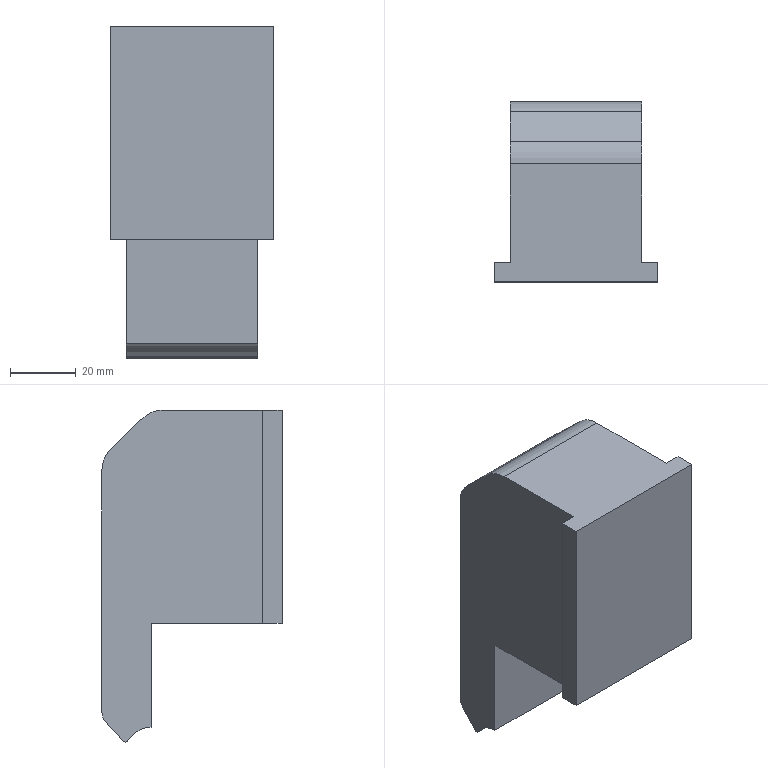Part | SolidWorks | features ICE 3, Extrusion 1, Fillet 1 | 1 solid | 21 faces | box 50 x 55 x 101.25 mm | volume 146000 mm3 | plane 14 | cylinder 7 | commonest cylinder face diameters 20 x2 21 x2 2 x1 10 x1 16.4 x1
STEP:
#1=CARTESIAN_POINT('',(10.5,25.,14.5));
#2=VERTEX_POINT('',#1);
#3=CARTESIAN_POINT('',(-10.5,25.,14.5));
#4=VERTEX_POINT('',#3);
#5=CARTESIAN_POINT('',(0.,25.,14.5));
#6=DIRECTION('',(0.,0.,-1.));
#7=DIRECTION('',(-1.,0.,0.));
#8=AXIS2_PLACEMENT_3D('',#5,#6,#7);
#9=CIRCLE('',#8,10.5);
#10=EDGE_CURVE('',#2,#4,#9,.T.);
#11=ORIENTED_EDGE('',*,*,#10,.F.);
#12=CARTESIAN_POINT('',(10.5,25.,-32.5));
#13=VERTEX_POINT('',#12);
#14=CARTESIAN_POINT('',(10.5,25.,14.5));
#15=DIRECTION('',(0.,0.,-1.));
#16=VECTOR('',#15,1000.);
#17=LINE('',#14,#16);
#18=EDGE_CURVE('',#2,#13,#17,.T.);
#19=ORIENTED_EDGE('',*,*,#18,.T.);
#20=CARTESIAN_POINT('',(-10.5,25.,-32.5));
#21=VERTEX_POINT('',#20);
#22=CARTESIAN_POINT('',(0.,25.,-32.5));
#23=DIRECTION('',(0.,0.,-1.));
#24=DIRECTION('',(-1.,0.,0.));
#25=AXIS2_PLACEMENT_3D('',#22,#23,#24);
#26=CIRCLE('',#25,10.5);
#27=EDGE_CURVE('',#13,#21,#26,.T.);
#28=ORIENTED_EDGE('',*,*,#27,.T.);
#29=CARTESIAN_POINT('',(-10.5,25.,14.5));
#30=DIRECTION('',(0.,0.,-1.));
#31=VECTOR('',#30,1000.);
#32=LINE('',#29,#31);
#33=EDGE_CURVE('',#4,#21,#32,.T.);
#34=ORIENTED_EDGE('',*,*,#33,.F.);
#35=EDGE_LOOP('',(#11,#19,#28,#34));
#36=FACE_OUTER_BOUND('',#35,.T.);
#37=CARTESIAN_POINT('',(0.,25.,14.5));
#38=DIRECTION('',(0.,0.,-1.));
#39=DIRECTION('',(-1.,0.,0.));
#40=AXIS2_PLACEMENT_3D('',#37,#38,#39);
#41=CYLINDRICAL_SURFACE('',#40,10.5);
#42=ADVANCED_FACE('',(#36),#41,.F.);
#43=CARTESIAN_POINT('',(20.,6.,32.5));
#44=VERTEX_POINT('',#43);
#45=CARTESIAN_POINT('',(20.,6.,-32.5));
#46=VERTEX_POINT('',#45);
#47=CARTESIAN_POINT('',(20.,6.,-32.5));
#48=DIRECTION('',(0.,0.,-1.));
#49=VECTOR('',#48,1000.);
#50=LINE('',#47,#49);
#51=EDGE_CURVE('',#44,#46,#50,.T.);
#52=ORIENTED_EDGE('',*,*,#51,.F.);
#53=CARTESIAN_POINT('',(25.,6.,32.5));
#54=VERTEX_POINT('',#53);
#55=CARTESIAN_POINT('',(-25.,6.,32.5));
#56=DIRECTION('',(1.,0.,0.));
#57=VECTOR('',#56,1000.);
#58=LINE('',#55,#57);
#59=EDGE_CURVE('',#44,#54,#58,.T.);
#60=ORIENTED_EDGE('',*,*,#59,.T.);
#61=CARTESIAN_POINT('',(25.,6.,-32.5));
#62=VERTEX_POINT('',#61);
#63=CARTESIAN_POINT('',(25.,6.,32.5));
#64=DIRECTION('',(0.,0.,-1.));
#65=VECTOR('',#64,1000.);
#66=LINE('',#63,#65);
#67=EDGE_CURVE('',#54,#62,#66,.T.);
#68=ORIENTED_EDGE('',*,*,#67,.T.);
#69=CARTESIAN_POINT('',(-25.,6.,-32.5));
#70=DIRECTION('',(-1.,0.,0.));
#71=VECTOR('',#70,1000.);
#72=LINE('',#69,#71);
#73=EDGE_CURVE('',#62,#46,#72,.T.);
#74=ORIENTED_EDGE('',*,*,#73,.T.);
#75=EDGE_LOOP('',(#52,#60,#68,#74));
#76=FACE_OUTER_BOUND('',#75,.T.);
#77=CARTESIAN_POINT('',(0.,6.,0.));
#78=DIRECTION('',(0.,-1.,0.));
#79=DIRECTION('',(0.,0.,-1.));
#80=AXIS2_PLACEMENT_3D('',#77,#78,#79);
#81=PLANE('',#80);
#82=ADVANCED_FACE('',(#76),#81,.F.);
#83=CARTESIAN_POINT('',(-20.,6.,-32.5));
#84=VERTEX_POINT('',#83);
#85=CARTESIAN_POINT('',(-20.,6.,32.5));
#86=VERTEX_POINT('',#85);
#87=CARTESIAN_POINT('',(-20.,6.,-32.5));
#88=DIRECTION('',(0.,0.,1.));
#89=VECTOR('',#88,1000.);
#90=LINE('',#87,#89);
#91=EDGE_CURVE('',#84,#86,#90,.T.);
#92=ORIENTED_EDGE('',*,*,#91,.F.);
#93=CARTESIAN_POINT('',(-25.,6.,-32.5));
#94=VERTEX_POINT('',#93);
#95=CARTESIAN_POINT('',(-25.,6.,-32.5));
#96=DIRECTION('',(-1.,0.,0.));
#97=VECTOR('',#96,1000.);
#98=LINE('',#95,#97);
#99=EDGE_CURVE('',#84,#94,#98,.T.);
#100=ORIENTED_EDGE('',*,*,#99,.T.);
#101=CARTESIAN_POINT('',(-25.,6.,32.5));
#102=VERTEX_POINT('',#101);
#103=CARTESIAN_POINT('',(-25.,6.,32.5));
#104=DIRECTION('',(0.,0.,1.));
#105=VECTOR('',#104,1000.);
#106=LINE('',#103,#105);
#107=EDGE_CURVE('',#94,#102,#106,.T.);
#108=ORIENTED_EDGE('',*,*,#107,.T.);
#109=CARTESIAN_POINT('',(-25.,6.,32.5));
#110=DIRECTION('',(1.,0.,0.));
#111=VECTOR('',#110,1000.);
#112=LINE('',#109,#111);
#113=EDGE_CURVE('',#102,#86,#112,.T.);
#114=ORIENTED_EDGE('',*,*,#113,.T.);
#115=EDGE_LOOP('',(#92,#100,#108,#114));
#116=FACE_OUTER_BOUND('',#115,.T.);
#117=CARTESIAN_POINT('',(0.,6.,0.));
#118=DIRECTION('',(0.,-1.,0.));
#119=DIRECTION('',(0.,0.,-1.));
#120=AXIS2_PLACEMENT_3D('',#117,#118,#119);
#121=PLANE('',#120);
#122=ADVANCED_FACE('',(#116),#121,.F.);
#123=CARTESIAN_POINT('',(25.,0.,32.5));
#124=VERTEX_POINT('',#123);
#125=CARTESIAN_POINT('',(25.,0.,-32.5));
#126=VERTEX_POINT('',#125);
#127=CARTESIAN_POINT('',(25.,0.,32.5));
#128=DIRECTION('',(0.,0.,-1.));
#129=VECTOR('',#128,1000.);
#130=LINE('',#127,#129);
#131=EDGE_CURVE('',#124,#126,#130,.T.);
#132=ORIENTED_EDGE('',*,*,#131,.T.);
#133=CARTESIAN_POINT('',(25.,6.,-32.5));
#134=DIRECTION('',(0.,-1.,0.));
#135=VECTOR('',#134,1000.);
#136=LINE('',#133,#135);
#137=EDGE_CURVE('',#62,#126,#136,.T.);
#138=ORIENTED_EDGE('',*,*,#137,.F.);
#139=ORIENTED_EDGE('',*,*,#67,.F.);
#140=CARTESIAN_POINT('',(25.,6.,32.5));
#141=DIRECTION('',(0.,-1.,0.));
#142=VECTOR('',#141,1000.);
#143=LINE('',#140,#142);
#144=EDGE_CURVE('',#54,#124,#143,.T.);
#145=ORIENTED_EDGE('',*,*,#144,.T.);
#146=EDGE_LOOP('',(#132,#138,#139,#145));
#147=FACE_OUTER_BOUND('',#146,.T.);
#148=CARTESIAN_POINT('',(25.,6.,32.5));
#149=DIRECTION('',(-1.,0.,0.));
#150=DIRECTION('',(0.,0.,1.));
#151=AXIS2_PLACEMENT_3D('',#148,#149,#150);
#152=PLANE('',#151);
#153=ADVANCED_FACE('',(#147),#152,.F.);
#154=CARTESIAN_POINT('',(0.,25.,-32.5));
#155=DIRECTION('',(0.,0.,-1.));
#156=DIRECTION('',(-1.,0.,0.));
#157=AXIS2_PLACEMENT_3D('',#154,#155,#156);
#158=CIRCLE('',#157,10.5);
#159=EDGE_CURVE('',#21,#13,#158,.T.);
#160=ORIENTED_EDGE('',*,*,#159,.F.);
#161=ORIENTED_EDGE('',*,*,#27,.F.);
#162=EDGE_LOOP('',(#160,#161));
#163=FACE_BOUND('',#162,.T.);
#164=CARTESIAN_POINT('',(-25.,0.,-32.5));
#165=VERTEX_POINT('',#164);
#166=CARTESIAN_POINT('',(-25.,0.,-32.5));
#167=DIRECTION('',(-1.,0.,0.));
#168=VECTOR('',#167,1000.);
#169=LINE('',#166,#168);
#170=EDGE_CURVE('',#126,#165,#169,.T.);
#171=ORIENTED_EDGE('',*,*,#170,.T.);
#172=CARTESIAN_POINT('',(-25.,6.,-32.5));
#173=DIRECTION('',(0.,-1.,0.));
#174=VECTOR('',#173,1000.);
#175=LINE('',#172,#174);
#176=EDGE_CURVE('',#94,#165,#175,.T.);
#177=ORIENTED_EDGE('',*,*,#176,.F.);
#178=ORIENTED_EDGE('',*,*,#99,.F.);
#179=CARTESIAN_POINT('',(-20.,40.,-32.5));
#180=VERTEX_POINT('',#179);
#181=CARTESIAN_POINT('',(-20.,40.,-32.5));
#182=DIRECTION('',(0.,-1.,0.));
#183=VECTOR('',#182,1000.);
#184=LINE('',#181,#183);
#185=EDGE_CURVE('',#180,#84,#184,.T.);
#186=ORIENTED_EDGE('',*,*,#185,.F.);
#187=CARTESIAN_POINT('',(20.,40.,-32.5));
#188=VERTEX_POINT('',#187);
#189=CARTESIAN_POINT('',(-20.,40.,-32.5));
#190=DIRECTION('',(-1.,0.,0.));
#191=VECTOR('',#190,1000.);
#192=LINE('',#189,#191);
#193=EDGE_CURVE('',#188,#180,#192,.T.);
#194=ORIENTED_EDGE('',*,*,#193,.F.);
#195=CARTESIAN_POINT('',(20.,40.,-32.5));
#196=DIRECTION('',(0.,-1.,0.));
#197=VECTOR('',#196,1000.);
#198=LINE('',#195,#197);
#199=EDGE_CURVE('',#188,#46,#198,.T.);
#200=ORIENTED_EDGE('',*,*,#199,.T.);
#201=ORIENTED_EDGE('',*,*,#73,.F.);
#202=ORIENTED_EDGE('',*,*,#137,.T.);
#203=EDGE_LOOP('',(#171,#177,#178,#186,#194,#200,#201,#202));
#204=FACE_OUTER_BOUND('',#203,.T.);
#205=CARTESIAN_POINT('',(-25.,6.,-32.5));
#206=DIRECTION('',(0.,0.,1.));
#207=DIRECTION('',(1.,0.,0.));
#208=AXIS2_PLACEMENT_3D('',#205,#206,#207);
#209=PLANE('',#208);
#210=ADVANCED_FACE('',(#163,#204),#209,.F.);
#211=CARTESIAN_POINT('',(-25.,0.,32.5));
#212=VERTEX_POINT('',#211);
#213=CARTESIAN_POINT('',(-25.,0.,32.5));
#214=DIRECTION('',(0.,0.,1.));
#215=VECTOR('',#214,1000.);
#216=LINE('',#213,#215);
#217=EDGE_CURVE('',#165,#212,#216,.T.);
#218=ORIENTED_EDGE('',*,*,#217,.T.);
#219=CARTESIAN_POINT('',(-25.,6.,32.5));
#220=DIRECTION('',(0.,-1.,0.));
#221=VECTOR('',#220,1000.);
#222=LINE('',#219,#221);
#223=EDGE_CURVE('',#102,#212,#222,.T.);
#224=ORIENTED_EDGE('',*,*,#223,.F.);
#225=ORIENTED_EDGE('',*,*,#107,.F.);
#226=ORIENTED_EDGE('',*,*,#176,.T.);
#227=EDGE_LOOP('',(#218,#224,#225,#226));
#228=FACE_OUTER_BOUND('',#227,.T.);
#229=CARTESIAN_POINT('',(-25.,6.,32.5));
#230=DIRECTION('',(1.,0.,0.));
#231=DIRECTION('',(0.,0.,-1.));
#232=AXIS2_PLACEMENT_3D('',#229,#230,#231);
#233=PLANE('',#232);
#234=ADVANCED_FACE('',(#228),#233,.F.);
#235=CARTESIAN_POINT('',(20.,36.004,32.5));
#236=VERTEX_POINT('',#235);
#237=CARTESIAN_POINT('',(20.,40.,32.5));
#238=DIRECTION('',(0.,-1.,0.));
#239=VECTOR('',#238,1000.);
#240=LINE('',#237,#239);
#241=EDGE_CURVE('',#236,#44,#240,.T.);
#242=ORIENTED_EDGE('',*,*,#241,.F.);
#243=CARTESIAN_POINT('',(-20.,36.004,32.5));
#244=VERTEX_POINT('',#243);
#245=CARTESIAN_POINT('',(-25.,36.004,32.5));
#246=DIRECTION('',(-1.,0.,0.));
#247=VECTOR('',#246,1000.);
#248=LINE('',#245,#247);
#249=EDGE_CURVE('',#236,#244,#248,.T.);
#250=ORIENTED_EDGE('',*,*,#249,.T.);
#251=CARTESIAN_POINT('',(-20.,40.,32.5));
#252=DIRECTION('',(0.,-1.,0.));
#253=VECTOR('',#252,1000.);
#254=LINE('',#251,#253);
#255=EDGE_CURVE('',#244,#86,#254,.T.);
#256=ORIENTED_EDGE('',*,*,#255,.T.);
#257=ORIENTED_EDGE('',*,*,#113,.F.);
#258=ORIENTED_EDGE('',*,*,#223,.T.);
#259=CARTESIAN_POINT('',(-25.,0.,32.5));
#260=DIRECTION('',(1.,0.,0.));
#261=VECTOR('',#260,1000.);
#262=LINE('',#259,#261);
#263=EDGE_CURVE('',#212,#124,#262,.T.);
#264=ORIENTED_EDGE('',*,*,#263,.T.);
#265=ORIENTED_EDGE('',*,*,#144,.F.);
#266=ORIENTED_EDGE('',*,*,#59,.F.);
#267=EDGE_LOOP('',(#242,#250,#256,#257,#258,#264,#265,#266));
#268=FACE_OUTER_BOUND('',#267,.T.);
#269=CARTESIAN_POINT('',(-25.,6.,32.5));
#270=DIRECTION('',(0.,0.,-1.));
#271=DIRECTION('',(-1.,0.,0.));
#272=AXIS2_PLACEMENT_3D('',#269,#270,#271);
#273=PLANE('',#272);
#274=ADVANCED_FACE('',(#268),#273,.F.);
#275=ORIENTED_EDGE('',*,*,#131,.F.);
#276=ORIENTED_EDGE('',*,*,#263,.F.);
#277=ORIENTED_EDGE('',*,*,#217,.F.);
#278=ORIENTED_EDGE('',*,*,#170,.F.);
#279=EDGE_LOOP('',(#275,#276,#277,#278));
#280=FACE_OUTER_BOUND('',#279,.T.);
#281=CARTESIAN_POINT('',(0.,0.,0.));
#282=DIRECTION('',(0.,-1.,0.));
#283=DIRECTION('',(0.,0.,-1.));
#284=AXIS2_PLACEMENT_3D('',#281,#282,#283);
#285=PLANE('',#284);
#286=ADVANCED_FACE('',(#280),#285,.T.);
#287=CARTESIAN_POINT('',(20.,55.,-59.535));
#288=VERTEX_POINT('',#287);
#289=CARTESIAN_POINT('',(20.,55.,13.946));
#290=VERTEX_POINT('',#289);
#291=CARTESIAN_POINT('',(20.,55.,-28.363));
#292=DIRECTION('',(0.,0.,1.));
#293=VECTOR('',#292,1000.);
#294=LINE('',#291,#293);
#295=EDGE_CURVE('',#288,#290,#294,.T.);
#296=ORIENTED_EDGE('',*,*,#295,.T.);
#297=CARTESIAN_POINT('',(20.,51.891,21.192));
#298=VERTEX_POINT('',#297);
#299=CARTESIAN_POINT('',(20.,45.,13.946));
#300=DIRECTION('',(1.,0.,0.));
#301=DIRECTION('',(0.,0.,1.));
#302=AXIS2_PLACEMENT_3D('',#299,#300,#301);
#303=CIRCLE('',#302,10.);
#304=EDGE_CURVE('',#290,#298,#303,.T.);
#305=ORIENTED_EDGE('',*,*,#304,.T.);
#306=CARTESIAN_POINT('',(20.,42.895,29.747));
#307=VERTEX_POINT('',#306);
#308=CARTESIAN_POINT('',(20.,55.,18.236));
#309=DIRECTION('',(0.,-0.7247,0.6891));
#310=VECTOR('',#309,1000.);
#311=LINE('',#308,#310);
#312=EDGE_CURVE('',#298,#307,#311,.T.);
#313=ORIENTED_EDGE('',*,*,#312,.T.);
#314=CARTESIAN_POINT('',(20.,36.004,22.5));
#315=DIRECTION('',(1.,0.,0.));
#316=DIRECTION('',(0.,0.,1.));
#317=AXIS2_PLACEMENT_3D('',#314,#315,#316);
#318=CIRCLE('',#317,10.);
#319=EDGE_CURVE('',#307,#236,#318,.T.);
#320=ORIENTED_EDGE('',*,*,#319,.T.);
#321=ORIENTED_EDGE('',*,*,#241,.T.);
#322=ORIENTED_EDGE('',*,*,#51,.T.);
#323=ORIENTED_EDGE('',*,*,#199,.F.);
#324=CARTESIAN_POINT('',(20.,40.,-64.3));
#325=VERTEX_POINT('',#324);
#326=CARTESIAN_POINT('',(20.,40.,32.5));
#327=DIRECTION('',(0.,0.,-1.));
#328=VECTOR('',#327,1000.);
#329=LINE('',#326,#328);
#330=EDGE_CURVE('',#188,#325,#329,.T.);
#331=ORIENTED_EDGE('',*,*,#330,.T.);
#332=CARTESIAN_POINT('',(20.,47.023,-68.266));
#333=VERTEX_POINT('',#332);
#334=CARTESIAN_POINT('',(20.,40.,-72.5));
#335=DIRECTION('',(-1.,0.,0.));
#336=DIRECTION('',(0.,0.,1.));
#337=AXIS2_PLACEMENT_3D('',#334,#335,#336);
#338=CIRCLE('',#337,8.2);
#339=EDGE_CURVE('',#325,#333,#338,.T.);
#340=ORIENTED_EDGE('',*,*,#339,.T.);
#341=CARTESIAN_POINT('',(20.,48.615,-68.427));
#342=VERTEX_POINT('',#341);
#343=CARTESIAN_POINT('',(20.,47.879,-67.75));
#344=DIRECTION('',(1.,0.,0.));
#345=DIRECTION('',(0.,0.,-1.));
#346=AXIS2_PLACEMENT_3D('',#343,#344,#345);
#347=CIRCLE('',#346,1.);
#348=EDGE_CURVE('',#333,#342,#347,.T.);
#349=ORIENTED_EDGE('',*,*,#348,.T.);
#350=CARTESIAN_POINT('',(20.,53.68,-62.92));
#351=VERTEX_POINT('',#350);
#352=CARTESIAN_POINT('',(20.,53.68,-62.92));
#353=DIRECTION('',(0.,0.677,0.736));
#354=VECTOR('',#353,1000.);
#355=LINE('',#352,#354);
#356=EDGE_CURVE('',#342,#351,#355,.T.);
#357=ORIENTED_EDGE('',*,*,#356,.T.);
#358=CARTESIAN_POINT('',(20.,50.,-59.535));
#359=DIRECTION('',(1.,0.,0.));
#360=DIRECTION('',(0.,0.,1.));
#361=AXIS2_PLACEMENT_3D('',#358,#359,#360);
#362=CIRCLE('',#361,5.);
#363=EDGE_CURVE('',#351,#288,#362,.T.);
#364=ORIENTED_EDGE('',*,*,#363,.T.);
#365=EDGE_LOOP('',(#296,#305,#313,#320,#321,#322,#323,#331,#340,#349,#357,#364));
#366=FACE_OUTER_BOUND('',#365,.T.);
#367=CARTESIAN_POINT('',(20.,40.,-32.5));
#368=DIRECTION('',(-1.,0.,0.));
#369=DIRECTION('',(0.,0.,1.));
#370=AXIS2_PLACEMENT_3D('',#367,#368,#369);
#371=PLANE('',#370);
#372=ADVANCED_FACE('',(#366),#371,.F.);
#373=CARTESIAN_POINT('',(-20.,51.891,21.192));
#374=VERTEX_POINT('',#373);
#375=CARTESIAN_POINT('',(-20.,42.895,29.747));
#376=VERTEX_POINT('',#375);
#377=CARTESIAN_POINT('',(-20.,55.,18.236));
#378=DIRECTION('',(0.,-0.7247,0.6891));
#379=VECTOR('',#378,1000.);
#380=LINE('',#377,#379);
#381=EDGE_CURVE('',#374,#376,#380,.T.);
#382=ORIENTED_EDGE('',*,*,#381,.F.);
#383=CARTESIAN_POINT('',(-20.,55.,13.946));
#384=VERTEX_POINT('',#383);
#385=CARTESIAN_POINT('',(-20.,45.,13.946));
#386=DIRECTION('',(-1.,0.,0.));
#387=DIRECTION('',(0.,0.,-1.));
#388=AXIS2_PLACEMENT_3D('',#385,#386,#387);
#389=CIRCLE('',#388,10.);
#390=EDGE_CURVE('',#374,#384,#389,.T.);
#391=ORIENTED_EDGE('',*,*,#390,.T.);
#392=CARTESIAN_POINT('',(-20.,55.,-59.535));
#393=VERTEX_POINT('',#392);
#394=CARTESIAN_POINT('',(-20.,55.,-28.363));
#395=DIRECTION('',(0.,0.,1.));
#396=VECTOR('',#395,1000.);
#397=LINE('',#394,#396);
#398=EDGE_CURVE('',#393,#384,#397,.T.);
#399=ORIENTED_EDGE('',*,*,#398,.F.);
#400=CARTESIAN_POINT('',(-20.,53.68,-62.92));
#401=VERTEX_POINT('',#400);
#402=CARTESIAN_POINT('',(-20.,50.,-59.535));
#403=DIRECTION('',(1.,0.,0.));
#404=DIRECTION('',(0.,0.,1.));
#405=AXIS2_PLACEMENT_3D('',#402,#403,#404);
#406=CIRCLE('',#405,5.);
#407=EDGE_CURVE('',#401,#393,#406,.T.);
#408=ORIENTED_EDGE('',*,*,#407,.F.);
#409=CARTESIAN_POINT('',(-20.,48.615,-68.427));
#410=VERTEX_POINT('',#409);
#411=CARTESIAN_POINT('',(-20.,53.68,-62.92));
#412=DIRECTION('',(0.,0.677,0.736));
#413=VECTOR('',#412,1000.);
#414=LINE('',#411,#413);
#415=EDGE_CURVE('',#410,#401,#414,.T.);
#416=ORIENTED_EDGE('',*,*,#415,.F.);
#417=CARTESIAN_POINT('',(-20.,47.023,-68.266));
#418=VERTEX_POINT('',#417);
#419=CARTESIAN_POINT('',(-20.,47.879,-67.75));
#420=DIRECTION('',(1.,0.,0.));
#421=DIRECTION('',(0.,0.,-1.));
#422=AXIS2_PLACEMENT_3D('',#419,#420,#421);
#423=CIRCLE('',#422,1.);
#424=EDGE_CURVE('',#418,#410,#423,.T.);
#425=ORIENTED_EDGE('',*,*,#424,.F.);
#426=CARTESIAN_POINT('',(-20.,40.,-64.3));
#427=VERTEX_POINT('',#426);
#428=CARTESIAN_POINT('',(-20.,40.,-72.5));
#429=DIRECTION('',(-1.,0.,0.));
#430=DIRECTION('',(0.,0.,1.));
#431=AXIS2_PLACEMENT_3D('',#428,#429,#430);
#432=CIRCLE('',#431,8.2);
#433=EDGE_CURVE('',#427,#418,#432,.T.);
#434=ORIENTED_EDGE('',*,*,#433,.F.);
#435=CARTESIAN_POINT('',(-20.,40.,32.5));
#436=DIRECTION('',(0.,0.,-1.));
#437=VECTOR('',#436,1000.);
#438=LINE('',#435,#437);
#439=EDGE_CURVE('',#180,#427,#438,.T.);
#440=ORIENTED_EDGE('',*,*,#439,.F.);
#441=ORIENTED_EDGE('',*,*,#185,.T.);
#442=ORIENTED_EDGE('',*,*,#91,.T.);
#443=ORIENTED_EDGE('',*,*,#255,.F.);
#444=CARTESIAN_POINT('',(-20.,36.004,22.5));
#445=DIRECTION('',(-1.,0.,0.));
#446=DIRECTION('',(0.,0.,-1.));
#447=AXIS2_PLACEMENT_3D('',#444,#445,#446);
#448=CIRCLE('',#447,10.);
#449=EDGE_CURVE('',#244,#376,#448,.T.);
#450=ORIENTED_EDGE('',*,*,#449,.T.);
#451=EDGE_LOOP('',(#382,#391,#399,#408,#416,#425,#434,#440,#441,#442,#443,#450));
#452=FACE_OUTER_BOUND('',#451,.T.);
#453=CARTESIAN_POINT('',(-20.,40.,-32.5));
#454=DIRECTION('',(1.,0.,0.));
#455=DIRECTION('',(0.,0.,-1.));
#456=AXIS2_PLACEMENT_3D('',#453,#454,#455);
#457=PLANE('',#456);
#458=ADVANCED_FACE('',(#452),#457,.F.);
#459=ORIENTED_EDGE('',*,*,#18,.F.);
#460=CARTESIAN_POINT('',(0.,25.,14.5));
#461=DIRECTION('',(0.,0.,-1.));
#462=DIRECTION('',(-1.,0.,0.));
#463=AXIS2_PLACEMENT_3D('',#460,#461,#462);
#464=CIRCLE('',#463,10.5);
#465=EDGE_CURVE('',#4,#2,#464,.T.);
#466=ORIENTED_EDGE('',*,*,#465,.F.);
#467=ORIENTED_EDGE('',*,*,#33,.T.);
#468=ORIENTED_EDGE('',*,*,#159,.T.);
#469=EDGE_LOOP('',(#459,#466,#467,#468));
#470=FACE_OUTER_BOUND('',#469,.T.);
#471=CARTESIAN_POINT('',(0.,25.,14.5));
#472=DIRECTION('',(0.,0.,-1.));
#473=DIRECTION('',(-1.,0.,0.));
#474=AXIS2_PLACEMENT_3D('',#471,#472,#473);
#475=CYLINDRICAL_SURFACE('',#474,10.5);
#476=ADVANCED_FACE('',(#470),#475,.F.);
#477=ORIENTED_EDGE('',*,*,#465,.T.);
#478=ORIENTED_EDGE('',*,*,#10,.T.);
#479=EDGE_LOOP('',(#477,#478));
#480=FACE_OUTER_BOUND('',#479,.T.);
#481=CARTESIAN_POINT('',(0.,25.,14.5));
#482=DIRECTION('',(0.,0.,-1.));
#483=DIRECTION('',(-1.,0.,0.));
#484=AXIS2_PLACEMENT_3D('',#481,#482,#483);
#485=PLANE('',#484);
#486=ADVANCED_FACE('',(#480),#485,.T.);
#487=ORIENTED_EDGE('',*,*,#330,.F.);
#488=ORIENTED_EDGE('',*,*,#193,.T.);
#489=ORIENTED_EDGE('',*,*,#439,.T.);
#490=CARTESIAN_POINT('',(20.,40.,-64.3));
#491=DIRECTION('',(-1.,0.,0.));
#492=VECTOR('',#491,1000.);
#493=LINE('',#490,#492);
#494=EDGE_CURVE('',#325,#427,#493,.T.);
#495=ORIENTED_EDGE('',*,*,#494,.F.);
#496=EDGE_LOOP('',(#487,#488,#489,#495));
#497=FACE_OUTER_BOUND('',#496,.T.);
#498=CARTESIAN_POINT('',(20.,40.,32.5));
#499=DIRECTION('',(0.,1.,0.));
#500=DIRECTION('',(0.,0.,1.));
#501=AXIS2_PLACEMENT_3D('',#498,#499,#500);
#502=PLANE('',#501);
#503=ADVANCED_FACE('',(#497),#502,.F.);
#504=ORIENTED_EDGE('',*,*,#312,.F.);
#505=CARTESIAN_POINT('',(20.,51.891,21.192));
#506=DIRECTION('',(-1.,0.,0.));
#507=VECTOR('',#506,1000.);
#508=LINE('',#505,#507);
#509=EDGE_CURVE('',#298,#374,#508,.T.);
#510=ORIENTED_EDGE('',*,*,#509,.T.);
#511=ORIENTED_EDGE('',*,*,#381,.T.);
#512=CARTESIAN_POINT('',(20.,42.895,29.747));
#513=DIRECTION('',(1.,0.,0.));
#514=VECTOR('',#513,1000.);
#515=LINE('',#512,#514);
#516=EDGE_CURVE('',#376,#307,#515,.T.);
#517=ORIENTED_EDGE('',*,*,#516,.T.);
#518=EDGE_LOOP('',(#504,#510,#511,#517));
#519=FACE_OUTER_BOUND('',#518,.T.);
#520=CARTESIAN_POINT('',(20.,55.,18.236));
#521=DIRECTION('',(0.,-0.6891,-0.7247));
#522=DIRECTION('',(0.,0.7247,-0.6891));
#523=AXIS2_PLACEMENT_3D('',#520,#521,#522);
#524=PLANE('',#523);
#525=ADVANCED_FACE('',(#519),#524,.F.);
#526=ORIENTED_EDGE('',*,*,#433,.T.);
#527=CARTESIAN_POINT('',(20.,47.023,-68.266));
#528=DIRECTION('',(-1.,0.,0.));
#529=VECTOR('',#528,1000.);
#530=LINE('',#527,#529);
#531=EDGE_CURVE('',#333,#418,#530,.T.);
#532=ORIENTED_EDGE('',*,*,#531,.F.);
#533=ORIENTED_EDGE('',*,*,#339,.F.);
#534=ORIENTED_EDGE('',*,*,#494,.T.);
#535=EDGE_LOOP('',(#526,#532,#533,#534));
#536=FACE_OUTER_BOUND('',#535,.T.);
#537=CARTESIAN_POINT('',(20.,40.,-72.5));
#538=DIRECTION('',(-1.,0.,0.));
#539=DIRECTION('',(0.,0.,1.));
#540=AXIS2_PLACEMENT_3D('',#537,#538,#539);
#541=CYLINDRICAL_SURFACE('',#540,8.2);
#542=ADVANCED_FACE('',(#536),#541,.F.);
#543=ORIENTED_EDGE('',*,*,#424,.T.);
#544=CARTESIAN_POINT('',(20.,48.615,-68.427));
#545=DIRECTION('',(-1.,0.,0.));
#546=VECTOR('',#545,1000.);
#547=LINE('',#544,#546);
#548=EDGE_CURVE('',#342,#410,#547,.T.);
#549=ORIENTED_EDGE('',*,*,#548,.F.);
#550=ORIENTED_EDGE('',*,*,#348,.F.);
#551=ORIENTED_EDGE('',*,*,#531,.T.);
#552=EDGE_LOOP('',(#543,#549,#550,#551));
#553=FACE_OUTER_BOUND('',#552,.T.);
#554=CARTESIAN_POINT('',(20.,47.879,-67.75));
#555=DIRECTION('',(-1.,0.,0.));
#556=DIRECTION('',(0.,0.,1.));
#557=AXIS2_PLACEMENT_3D('',#554,#555,#556);
#558=CYLINDRICAL_SURFACE('',#557,1.);
#559=ADVANCED_FACE('',(#553),#558,.T.);
#560=ORIENTED_EDGE('',*,*,#415,.T.);
#561=CARTESIAN_POINT('',(20.,53.68,-62.92));
#562=DIRECTION('',(-1.,0.,0.));
#563=VECTOR('',#562,1000.);
#564=LINE('',#561,#563);
#565=EDGE_CURVE('',#351,#401,#564,.T.);
#566=ORIENTED_EDGE('',*,*,#565,.F.);
#567=ORIENTED_EDGE('',*,*,#356,.F.);
#568=ORIENTED_EDGE('',*,*,#548,.T.);
#569=EDGE_LOOP('',(#560,#566,#567,#568));
#570=FACE_OUTER_BOUND('',#569,.T.);
#571=CARTESIAN_POINT('',(20.,53.68,-62.92));
#572=DIRECTION('',(0.,-0.736,0.677));
#573=DIRECTION('',(0.,-0.677,-0.736));
#574=AXIS2_PLACEMENT_3D('',#571,#572,#573);
#575=PLANE('',#574);
#576=ADVANCED_FACE('',(#570),#575,.F.);
#577=ORIENTED_EDGE('',*,*,#407,.T.);
#578=CARTESIAN_POINT('',(20.,55.,-59.535));
#579=DIRECTION('',(-1.,0.,0.));
#580=VECTOR('',#579,1000.);
#581=LINE('',#578,#580);
#582=EDGE_CURVE('',#288,#393,#581,.T.);
#583=ORIENTED_EDGE('',*,*,#582,.F.);
#584=ORIENTED_EDGE('',*,*,#363,.F.);
#585=ORIENTED_EDGE('',*,*,#565,.T.);
#586=EDGE_LOOP('',(#577,#583,#584,#585));
#587=FACE_OUTER_BOUND('',#586,.T.);
#588=CARTESIAN_POINT('',(20.,50.,-59.535));
#589=DIRECTION('',(-1.,0.,0.));
#590=DIRECTION('',(0.,0.,1.));
#591=AXIS2_PLACEMENT_3D('',#588,#589,#590);
#592=CYLINDRICAL_SURFACE('',#591,5.);
#593=ADVANCED_FACE('',(#587),#592,.T.);
#594=ORIENTED_EDGE('',*,*,#398,.T.);
#595=CARTESIAN_POINT('',(20.,55.,13.946));
#596=DIRECTION('',(1.,0.,0.));
#597=VECTOR('',#596,1000.);
#598=LINE('',#595,#597);
#599=EDGE_CURVE('',#384,#290,#598,.T.);
#600=ORIENTED_EDGE('',*,*,#599,.T.);
#601=ORIENTED_EDGE('',*,*,#295,.F.);
#602=ORIENTED_EDGE('',*,*,#582,.T.);
#603=EDGE_LOOP('',(#594,#600,#601,#602));
#604=FACE_OUTER_BOUND('',#603,.T.);
#605=CARTESIAN_POINT('',(20.,55.,-28.363));
#606=DIRECTION('',(0.,-1.,0.));
#607=DIRECTION('',(0.,0.,-1.));
#608=AXIS2_PLACEMENT_3D('',#605,#606,#607);
#609=PLANE('',#608);
#610=ADVANCED_FACE('',(#604),#609,.F.);
#611=ORIENTED_EDGE('',*,*,#304,.F.);
#612=ORIENTED_EDGE('',*,*,#599,.F.);
#613=ORIENTED_EDGE('',*,*,#390,.F.);
#614=ORIENTED_EDGE('',*,*,#509,.F.);
#615=EDGE_LOOP('',(#611,#612,#613,#614));
#616=FACE_OUTER_BOUND('',#615,.T.);
#617=CARTESIAN_POINT('',(20.,45.,13.946));
#618=DIRECTION('',(-1.,0.,0.));
#619=DIRECTION('',(0.,0.,1.));
#620=AXIS2_PLACEMENT_3D('',#617,#618,#619);
#621=CYLINDRICAL_SURFACE('',#620,10.);
#622=ADVANCED_FACE('',(#616),#621,.T.);
#623=ORIENTED_EDGE('',*,*,#449,.F.);
#624=ORIENTED_EDGE('',*,*,#249,.F.);
#625=ORIENTED_EDGE('',*,*,#319,.F.);
#626=ORIENTED_EDGE('',*,*,#516,.F.);
#627=EDGE_LOOP('',(#623,#624,#625,#626));
#628=FACE_OUTER_BOUND('',#627,.T.);
#629=CARTESIAN_POINT('',(20.,36.004,22.5));
#630=DIRECTION('',(1.,0.,0.));
#631=DIRECTION('',(0.,0.,-1.));
#632=AXIS2_PLACEMENT_3D('',#629,#630,#631);
#633=CYLINDRICAL_SURFACE('',#632,10.);
#634=ADVANCED_FACE('',(#628),#633,.T.);
#635=CLOSED_SHELL('',(#42,#82,#122,#153,#210,#234,#274,#286,#372,#458,#476,#486,#503,#525,#542,#559,#576,#593,#610,#622,#634));
#636=MANIFOLD_SOLID_BREP('',#635);
#637=CARTESIAN_POINT('',(0.,0.,0.));
#638=DIRECTION('',(0.,0.,1.));
#639=DIRECTION('',(1.,0.,0.));
#640=AXIS2_PLACEMENT_3D('',#637,#638,#639);
#641=(LENGTH_UNIT()NAMED_UNIT(*)SI_UNIT(.MILLI.,.METRE.));
#642=UNCERTAINTY_MEASURE_WITH_UNIT(LENGTH_MEASURE(0.00001),#641,'','');
#643=(NAMED_UNIT(*)PLANE_ANGLE_UNIT()SI_UNIT($,.RADIAN.));
#644=(NAMED_UNIT(*)SI_UNIT($,.STERADIAN.)SOLID_ANGLE_UNIT());
#645=(GEOMETRIC_REPRESENTATION_CONTEXT(3)GLOBAL_UNCERTAINTY_ASSIGNED_CONTEXT((#642))GLOBAL_UNIT_ASSIGNED_CONTEXT((#641,#643,#644))REPRESENTATION_CONTEXT('',''));
#646=ADVANCED_BREP_SHAPE_REPRESENTATION('',(#636,#640),#645);